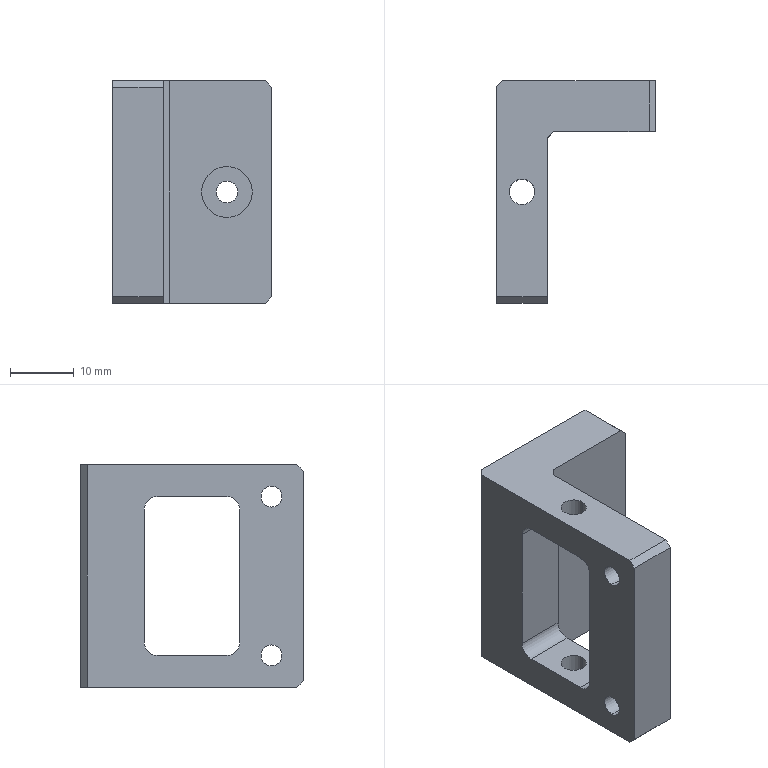Part | SolidWorks | features ICE 3, HoleWzd 2, Chamfer 1, Extrusion 1, Fillet 1 | 1 solid | 38 faces | box 25 x 35 x 35 mm | volume 11031 mm3 | plane 20 | cylinder 18 | commonest cylinder face diameters 4 x8 3.3 x4 3.4 x2 6.5 x2 8 x2
STEP:
#1=CARTESIAN_POINT('',(18.,31.6,-3.25));
#2=VERTEX_POINT('',#1);
#3=CARTESIAN_POINT('',(18.,31.6,3.25));
#4=VERTEX_POINT('',#3);
#5=CARTESIAN_POINT('',(18.,31.6,0.));
#6=DIRECTION('',(0.,1.,0.));
#7=DIRECTION('',(0.,0.,1.));
#8=AXIS2_PLACEMENT_3D('',#5,#6,#7);
#9=CIRCLE('',#8,3.25);
#10=EDGE_CURVE('',#2,#4,#9,.T.);
#11=ORIENTED_EDGE('',*,*,#10,.F.);
#12=CARTESIAN_POINT('',(18.,35.,-3.25));
#13=VERTEX_POINT('',#12);
#14=CARTESIAN_POINT('',(18.,35.,-3.25));
#15=DIRECTION('',(0.,1.,0.));
#16=VECTOR('',#15,1000.);
#17=LINE('',#14,#16);
#18=EDGE_CURVE('',#2,#13,#17,.T.);
#19=ORIENTED_EDGE('',*,*,#18,.T.);
#20=CARTESIAN_POINT('',(18.,35.,3.25));
#21=VERTEX_POINT('',#20);
#22=CARTESIAN_POINT('',(18.,35.,0.));
#23=DIRECTION('',(0.,1.,0.));
#24=DIRECTION('',(0.,0.,1.));
#25=AXIS2_PLACEMENT_3D('',#22,#23,#24);
#26=CIRCLE('',#25,3.25);
#27=EDGE_CURVE('',#13,#21,#26,.T.);
#28=ORIENTED_EDGE('',*,*,#27,.T.);
#29=CARTESIAN_POINT('',(18.,35.,3.25));
#30=DIRECTION('',(0.,1.,0.));
#31=VECTOR('',#30,1000.);
#32=LINE('',#29,#31);
#33=EDGE_CURVE('',#4,#21,#32,.T.);
#34=ORIENTED_EDGE('',*,*,#33,.F.);
#35=EDGE_LOOP('',(#11,#19,#28,#34));
#36=FACE_OUTER_BOUND('',#35,.T.);
#37=CARTESIAN_POINT('',(18.,35.,0.));
#38=DIRECTION('',(0.,1.,0.));
#39=DIRECTION('',(0.,0.,1.));
#40=AXIS2_PLACEMENT_3D('',#37,#38,#39);
#41=CYLINDRICAL_SURFACE('',#40,3.25);
#42=ADVANCED_FACE('',(#36),#41,.F.);
#43=CARTESIAN_POINT('',(18.,30.,1.7));
#44=VERTEX_POINT('',#43);
#45=CARTESIAN_POINT('',(18.,30.,-1.7));
#46=VERTEX_POINT('',#45);
#47=CARTESIAN_POINT('',(18.,30.,0.));
#48=DIRECTION('',(0.,-1.,0.));
#49=DIRECTION('',(1.,0.,0.));
#50=AXIS2_PLACEMENT_3D('',#47,#48,#49);
#51=CIRCLE('',#50,1.7);
#52=EDGE_CURVE('',#44,#46,#51,.T.);
#53=ORIENTED_EDGE('',*,*,#52,.T.);
#54=CARTESIAN_POINT('',(18.,31.6,-1.7));
#55=VERTEX_POINT('',#54);
#56=CARTESIAN_POINT('',(18.,35.,-1.7));
#57=DIRECTION('',(0.,1.,0.));
#58=VECTOR('',#57,1000.);
#59=LINE('',#56,#58);
#60=EDGE_CURVE('',#46,#55,#59,.T.);
#61=ORIENTED_EDGE('',*,*,#60,.T.);
#62=CARTESIAN_POINT('',(18.,31.6,1.7));
#63=VERTEX_POINT('',#62);
#64=CARTESIAN_POINT('',(18.,31.6,0.));
#65=DIRECTION('',(0.,1.,0.));
#66=DIRECTION('',(0.,0.,1.));
#67=AXIS2_PLACEMENT_3D('',#64,#65,#66);
#68=CIRCLE('',#67,1.7);
#69=EDGE_CURVE('',#55,#63,#68,.T.);
#70=ORIENTED_EDGE('',*,*,#69,.T.);
#71=CARTESIAN_POINT('',(18.,35.,1.7));
#72=DIRECTION('',(0.,1.,0.));
#73=VECTOR('',#72,1000.);
#74=LINE('',#71,#73);
#75=EDGE_CURVE('',#44,#63,#74,.T.);
#76=ORIENTED_EDGE('',*,*,#75,.F.);
#77=EDGE_LOOP('',(#53,#61,#70,#76));
#78=FACE_OUTER_BOUND('',#77,.T.);
#79=CARTESIAN_POINT('',(18.,35.,0.));
#80=DIRECTION('',(0.,1.,0.));
#81=DIRECTION('',(0.,0.,1.));
#82=AXIS2_PLACEMENT_3D('',#79,#80,#81);
#83=CYLINDRICAL_SURFACE('',#82,1.7);
#84=ADVANCED_FACE('',(#78),#83,.F.);
#85=CARTESIAN_POINT('',(14.,30.,0.));
#86=VERTEX_POINT('',#85);
#87=CARTESIAN_POINT('',(22.,30.,0.));
#88=VERTEX_POINT('',#87);
#89=CARTESIAN_POINT('',(18.,30.,0.));
#90=DIRECTION('',(0.,-1.,0.));
#91=DIRECTION('',(1.,0.,0.));
#92=AXIS2_PLACEMENT_3D('',#89,#90,#91);
#93=CIRCLE('',#92,4.);
#94=EDGE_CURVE('',#86,#88,#93,.T.);
#95=ORIENTED_EDGE('',*,*,#94,.F.);
#96=CARTESIAN_POINT('',(14.,27.,0.));
#97=VERTEX_POINT('',#96);
#98=CARTESIAN_POINT('',(14.,30.,0.));
#99=DIRECTION('',(0.,-1.,0.));
#100=VECTOR('',#99,1000.);
#101=LINE('',#98,#100);
#102=EDGE_CURVE('',#86,#97,#101,.T.);
#103=ORIENTED_EDGE('',*,*,#102,.T.);
#104=CARTESIAN_POINT('',(22.,27.,0.));
#105=VERTEX_POINT('',#104);
#106=CARTESIAN_POINT('',(18.,27.,0.));
#107=DIRECTION('',(0.,-1.,0.));
#108=DIRECTION('',(1.,0.,0.));
#109=AXIS2_PLACEMENT_3D('',#106,#107,#108);
#110=CIRCLE('',#109,4.);
#111=EDGE_CURVE('',#97,#105,#110,.T.);
#112=ORIENTED_EDGE('',*,*,#111,.T.);
#113=CARTESIAN_POINT('',(22.,30.,0.));
#114=DIRECTION('',(0.,-1.,0.));
#115=VECTOR('',#114,1000.);
#116=LINE('',#113,#115);
#117=EDGE_CURVE('',#88,#105,#116,.T.);
#118=ORIENTED_EDGE('',*,*,#117,.F.);
#119=EDGE_LOOP('',(#95,#103,#112,#118));
#120=FACE_OUTER_BOUND('',#119,.T.);
#121=CARTESIAN_POINT('',(18.,30.,0.));
#122=DIRECTION('',(0.,-1.,0.));
#123=DIRECTION('',(1.,0.,0.));
#124=AXIS2_PLACEMENT_3D('',#121,#122,#123);
#125=CYLINDRICAL_SURFACE('',#124,4.);
#126=ADVANCED_FACE('',(#120),#125,.F.);
#127=CARTESIAN_POINT('',(2.,17.5,-17.5));
#128=VERTEX_POINT('',#127);
#129=CARTESIAN_POINT('',(6.,17.5,-17.5));
#130=VERTEX_POINT('',#129);
#131=CARTESIAN_POINT('',(4.,17.5,-17.5));
#132=DIRECTION('',(0.,0.,1.));
#133=DIRECTION('',(1.,0.,0.));
#134=AXIS2_PLACEMENT_3D('',#131,#132,#133);
#135=CIRCLE('',#134,2.);
#136=EDGE_CURVE('',#128,#130,#135,.T.);
#137=ORIENTED_EDGE('',*,*,#136,.F.);
#138=CARTESIAN_POINT('',(2.,17.5,-12.5));
#139=VERTEX_POINT('',#138);
#140=CARTESIAN_POINT('',(2.,17.5,-17.5));
#141=DIRECTION('',(0.,0.,1.));
#142=VECTOR('',#141,1000.);
#143=LINE('',#140,#142);
#144=EDGE_CURVE('',#128,#139,#143,.T.);
#145=ORIENTED_EDGE('',*,*,#144,.T.);
#146=CARTESIAN_POINT('',(6.,17.5,-12.5));
#147=VERTEX_POINT('',#146);
#148=CARTESIAN_POINT('',(4.,17.5,-12.5));
#149=DIRECTION('',(0.,0.,-1.));
#150=DIRECTION('',(-1.,0.,0.));
#151=AXIS2_PLACEMENT_3D('',#148,#149,#150);
#152=CIRCLE('',#151,2.);
#153=EDGE_CURVE('',#147,#139,#152,.T.);
#154=ORIENTED_EDGE('',*,*,#153,.F.);
#155=CARTESIAN_POINT('',(6.,17.5,-17.5));
#156=DIRECTION('',(0.,0.,1.));
#157=VECTOR('',#156,1000.);
#158=LINE('',#155,#157);
#159=EDGE_CURVE('',#130,#147,#158,.T.);
#160=ORIENTED_EDGE('',*,*,#159,.F.);
#161=EDGE_LOOP('',(#137,#145,#154,#160));
#162=FACE_OUTER_BOUND('',#161,.T.);
#163=CARTESIAN_POINT('',(4.,17.5,-17.5));
#164=DIRECTION('',(0.,0.,1.));
#165=DIRECTION('',(1.,0.,0.));
#166=AXIS2_PLACEMENT_3D('',#163,#164,#165);
#167=CYLINDRICAL_SURFACE('',#166,2.);
#168=ADVANCED_FACE('',(#162),#167,.F.);
#169=CARTESIAN_POINT('',(2.,17.5,12.5));
#170=VERTEX_POINT('',#169);
#171=CARTESIAN_POINT('',(6.,17.5,12.5));
#172=VERTEX_POINT('',#171);
#173=CARTESIAN_POINT('',(4.,17.5,12.5));
#174=DIRECTION('',(0.,0.,1.));
#175=DIRECTION('',(0.,-1.,0.));
#176=AXIS2_PLACEMENT_3D('',#173,#174,#175);
#177=CIRCLE('',#176,2.);
#178=EDGE_CURVE('',#170,#172,#177,.T.);
#179=ORIENTED_EDGE('',*,*,#178,.F.);
#180=CARTESIAN_POINT('',(2.,17.5,17.5));
#181=VERTEX_POINT('',#180);
#182=CARTESIAN_POINT('',(2.,17.5,-17.5));
#183=DIRECTION('',(0.,0.,1.));
#184=VECTOR('',#183,1000.);
#185=LINE('',#182,#184);
#186=EDGE_CURVE('',#170,#181,#185,.T.);
#187=ORIENTED_EDGE('',*,*,#186,.T.);
#188=CARTESIAN_POINT('',(6.,17.5,17.5));
#189=VERTEX_POINT('',#188);
#190=CARTESIAN_POINT('',(4.,17.5,17.5));
#191=DIRECTION('',(0.,0.,1.));
#192=DIRECTION('',(1.,0.,0.));
#193=AXIS2_PLACEMENT_3D('',#190,#191,#192);
#194=CIRCLE('',#193,2.);
#195=EDGE_CURVE('',#181,#189,#194,.T.);
#196=ORIENTED_EDGE('',*,*,#195,.T.);
#197=CARTESIAN_POINT('',(6.,17.5,-17.5));
#198=DIRECTION('',(0.,0.,1.));
#199=VECTOR('',#198,1000.);
#200=LINE('',#197,#199);
#201=EDGE_CURVE('',#172,#189,#200,.T.);
#202=ORIENTED_EDGE('',*,*,#201,.F.);
#203=EDGE_LOOP('',(#179,#187,#196,#202));
#204=FACE_OUTER_BOUND('',#203,.T.);
#205=CARTESIAN_POINT('',(4.,17.5,-17.5));
#206=DIRECTION('',(0.,0.,1.));
#207=DIRECTION('',(1.,0.,0.));
#208=AXIS2_PLACEMENT_3D('',#205,#206,#207);
#209=CYLINDRICAL_SURFACE('',#208,2.);
#210=ADVANCED_FACE('',(#204),#209,.F.);
#211=CARTESIAN_POINT('',(8.,5.,-14.15));
#212=VERTEX_POINT('',#211);
#213=CARTESIAN_POINT('',(8.,5.,-10.85));
#214=VERTEX_POINT('',#213);
#215=CARTESIAN_POINT('',(8.,5.,-12.5));
#216=DIRECTION('',(-1.,0.,0.));
#217=DIRECTION('',(0.,-1.,0.));
#218=AXIS2_PLACEMENT_3D('',#215,#216,#217);
#219=CIRCLE('',#218,1.65);
#220=EDGE_CURVE('',#212,#214,#219,.T.);
#221=ORIENTED_EDGE('',*,*,#220,.F.);
#222=CARTESIAN_POINT('',(0.,5.,-14.15));
#223=VERTEX_POINT('',#222);
#224=CARTESIAN_POINT('',(0.,5.,-14.15));
#225=DIRECTION('',(-1.,0.,0.));
#226=VECTOR('',#225,1000.);
#227=LINE('',#224,#226);
#228=EDGE_CURVE('',#212,#223,#227,.T.);
#229=ORIENTED_EDGE('',*,*,#228,.T.);
#230=CARTESIAN_POINT('',(0.,5.,-10.85));
#231=VERTEX_POINT('',#230);
#232=CARTESIAN_POINT('',(0.,5.,-12.5));
#233=DIRECTION('',(-1.,0.,0.));
#234=DIRECTION('',(0.,0.,1.));
#235=AXIS2_PLACEMENT_3D('',#232,#233,#234);
#236=CIRCLE('',#235,1.65);
#237=EDGE_CURVE('',#223,#231,#236,.T.);
#238=ORIENTED_EDGE('',*,*,#237,.T.);
#239=CARTESIAN_POINT('',(0.,5.,-10.85));
#240=DIRECTION('',(-1.,0.,0.));
#241=VECTOR('',#240,1000.);
#242=LINE('',#239,#241);
#243=EDGE_CURVE('',#214,#231,#242,.T.);
#244=ORIENTED_EDGE('',*,*,#243,.F.);
#245=EDGE_LOOP('',(#221,#229,#238,#244));
#246=FACE_OUTER_BOUND('',#245,.T.);
#247=CARTESIAN_POINT('',(0.,5.,-12.5));
#248=DIRECTION('',(-1.,0.,0.));
#249=DIRECTION('',(0.,0.,1.));
#250=AXIS2_PLACEMENT_3D('',#247,#248,#249);
#251=CYLINDRICAL_SURFACE('',#250,1.65);
#252=ADVANCED_FACE('',(#246),#251,.F.);
#253=CARTESIAN_POINT('',(8.,5.,10.85));
#254=VERTEX_POINT('',#253);
#255=CARTESIAN_POINT('',(8.,5.,14.15));
#256=VERTEX_POINT('',#255);
#257=CARTESIAN_POINT('',(8.,5.,12.5));
#258=DIRECTION('',(-1.,0.,0.));
#259=DIRECTION('',(0.,-1.,0.));
#260=AXIS2_PLACEMENT_3D('',#257,#258,#259);
#261=CIRCLE('',#260,1.65);
#262=EDGE_CURVE('',#254,#256,#261,.T.);
#263=ORIENTED_EDGE('',*,*,#262,.F.);
#264=CARTESIAN_POINT('',(0.,5.,10.85));
#265=VERTEX_POINT('',#264);
#266=CARTESIAN_POINT('',(0.,5.,10.85));
#267=DIRECTION('',(-1.,0.,0.));
#268=VECTOR('',#267,1000.);
#269=LINE('',#266,#268);
#270=EDGE_CURVE('',#254,#265,#269,.T.);
#271=ORIENTED_EDGE('',*,*,#270,.T.);
#272=CARTESIAN_POINT('',(0.,5.,14.15));
#273=VERTEX_POINT('',#272);
#274=CARTESIAN_POINT('',(0.,5.,12.5));
#275=DIRECTION('',(-1.,0.,0.));
#276=DIRECTION('',(0.,0.,1.));
#277=AXIS2_PLACEMENT_3D('',#274,#275,#276);
#278=CIRCLE('',#277,1.65);
#279=EDGE_CURVE('',#265,#273,#278,.T.);
#280=ORIENTED_EDGE('',*,*,#279,.T.);
#281=CARTESIAN_POINT('',(0.,5.,14.15));
#282=DIRECTION('',(-1.,0.,0.));
#283=VECTOR('',#282,1000.);
#284=LINE('',#281,#283);
#285=EDGE_CURVE('',#256,#273,#284,.T.);
#286=ORIENTED_EDGE('',*,*,#285,.F.);
#287=EDGE_LOOP('',(#263,#271,#280,#286));
#288=FACE_OUTER_BOUND('',#287,.T.);
#289=CARTESIAN_POINT('',(0.,5.,12.5));
#290=DIRECTION('',(-1.,0.,0.));
#291=DIRECTION('',(0.,0.,1.));
#292=AXIS2_PLACEMENT_3D('',#289,#290,#291);
#293=CYLINDRICAL_SURFACE('',#292,1.65);
#294=ADVANCED_FACE('',(#288),#293,.F.);
#295=CARTESIAN_POINT('',(0.,0.,16.5));
#296=VERTEX_POINT('',#295);
#297=CARTESIAN_POINT('',(0.,0.,-16.5));
#298=VERTEX_POINT('',#297);
#299=CARTESIAN_POINT('',(0.,0.,17.5));
#300=DIRECTION('',(0.,0.,-1.));
#301=VECTOR('',#300,1000.);
#302=LINE('',#299,#301);
#303=EDGE_CURVE('',#296,#298,#302,.T.);
#304=ORIENTED_EDGE('',*,*,#303,.T.);
#305=CARTESIAN_POINT('',(8.,0.,-16.5));
#306=VERTEX_POINT('',#305);
#307=CARTESIAN_POINT('',(8.,0.,-16.5));
#308=DIRECTION('',(1.,0.,0.));
#309=VECTOR('',#308,1000.);
#310=LINE('',#307,#309);
#311=EDGE_CURVE('',#298,#306,#310,.T.);
#312=ORIENTED_EDGE('',*,*,#311,.T.);
#313=CARTESIAN_POINT('',(8.,0.,16.5));
#314=VERTEX_POINT('',#313);
#315=CARTESIAN_POINT('',(8.,0.,17.5));
#316=DIRECTION('',(0.,0.,-1.));
#317=VECTOR('',#316,1000.);
#318=LINE('',#315,#317);
#319=EDGE_CURVE('',#314,#306,#318,.T.);
#320=ORIENTED_EDGE('',*,*,#319,.F.);
#321=CARTESIAN_POINT('',(8.,0.,16.5));
#322=DIRECTION('',(-1.,0.,0.));
#323=VECTOR('',#322,1000.);
#324=LINE('',#321,#323);
#325=EDGE_CURVE('',#314,#296,#324,.T.);
#326=ORIENTED_EDGE('',*,*,#325,.T.);
#327=EDGE_LOOP('',(#304,#312,#320,#326));
#328=FACE_OUTER_BOUND('',#327,.T.);
#329=CARTESIAN_POINT('',(8.,0.,17.5));
#330=DIRECTION('',(0.,1.,0.));
#331=DIRECTION('',(-1.,0.,0.));
#332=AXIS2_PLACEMENT_3D('',#329,#330,#331);
#333=PLANE('',#332);
#334=ADVANCED_FACE('',(#328),#333,.F.);
#335=CARTESIAN_POINT('',(8.,5.,-12.5));
#336=DIRECTION('',(-1.,0.,0.));
#337=DIRECTION('',(0.,-1.,0.));
#338=AXIS2_PLACEMENT_3D('',#335,#336,#337);
#339=CIRCLE('',#338,1.65);
#340=EDGE_CURVE('',#214,#212,#339,.T.);
#341=ORIENTED_EDGE('',*,*,#340,.T.);
#342=ORIENTED_EDGE('',*,*,#220,.T.);
#343=EDGE_LOOP('',(#341,#342));
#344=FACE_BOUND('',#343,.T.);
#345=CARTESIAN_POINT('',(8.,5.,12.5));
#346=DIRECTION('',(-1.,0.,0.));
#347=DIRECTION('',(0.,-1.,0.));
#348=AXIS2_PLACEMENT_3D('',#345,#346,#347);
#349=CIRCLE('',#348,1.65);
#350=EDGE_CURVE('',#256,#254,#349,.T.);
#351=ORIENTED_EDGE('',*,*,#350,.T.);
#352=ORIENTED_EDGE('',*,*,#262,.T.);
#353=EDGE_LOOP('',(#351,#352));
#354=FACE_BOUND('',#353,.T.);
#355=CARTESIAN_POINT('',(8.,12.,12.5));
#356=VERTEX_POINT('',#355);
#357=CARTESIAN_POINT('',(8.,23.,12.5));
#358=VERTEX_POINT('',#357);
#359=CARTESIAN_POINT('',(8.,27.,12.5));
#360=DIRECTION('',(0.,1.,0.));
#361=VECTOR('',#360,1000.);
#362=LINE('',#359,#361);
#363=EDGE_CURVE('',#356,#358,#362,.T.);
#364=ORIENTED_EDGE('',*,*,#363,.T.);
#365=CARTESIAN_POINT('',(8.,25.,10.5));
#366=VERTEX_POINT('',#365);
#367=CARTESIAN_POINT('',(8.,23.,10.5));
#368=DIRECTION('',(-1.,0.,0.));
#369=DIRECTION('',(0.,-1.,0.));
#370=AXIS2_PLACEMENT_3D('',#367,#368,#369);
#371=CIRCLE('',#370,2.);
#372=EDGE_CURVE('',#358,#366,#371,.T.);
#373=ORIENTED_EDGE('',*,*,#372,.T.);
#374=CARTESIAN_POINT('',(8.,25.,-10.5));
#375=VERTEX_POINT('',#374);
#376=CARTESIAN_POINT('',(8.,25.,17.5));
#377=DIRECTION('',(0.,0.,-1.));
#378=VECTOR('',#377,1000.);
#379=LINE('',#376,#378);
#380=EDGE_CURVE('',#366,#375,#379,.T.);
#381=ORIENTED_EDGE('',*,*,#380,.T.);
#382=CARTESIAN_POINT('',(8.,23.,-12.5));
#383=VERTEX_POINT('',#382);
#384=CARTESIAN_POINT('',(8.,23.,-10.5));
#385=DIRECTION('',(-1.,0.,0.));
#386=DIRECTION('',(0.,-1.,0.));
#387=AXIS2_PLACEMENT_3D('',#384,#385,#386);
#388=CIRCLE('',#387,2.);
#389=EDGE_CURVE('',#375,#383,#388,.T.);
#390=ORIENTED_EDGE('',*,*,#389,.T.);
#391=CARTESIAN_POINT('',(8.,12.,-12.5));
#392=VERTEX_POINT('',#391);
#393=CARTESIAN_POINT('',(8.,27.,-12.5));
#394=DIRECTION('',(0.,-1.,0.));
#395=VECTOR('',#394,1000.);
#396=LINE('',#393,#395);
#397=EDGE_CURVE('',#383,#392,#396,.T.);
#398=ORIENTED_EDGE('',*,*,#397,.T.);
#399=CARTESIAN_POINT('',(8.,10.,-10.5));
#400=VERTEX_POINT('',#399);
#401=CARTESIAN_POINT('',(8.,12.,-10.5));
#402=DIRECTION('',(-1.,0.,0.));
#403=DIRECTION('',(0.,-1.,0.));
#404=AXIS2_PLACEMENT_3D('',#401,#402,#403);
#405=CIRCLE('',#404,2.);
#406=EDGE_CURVE('',#392,#400,#405,.T.);
#407=ORIENTED_EDGE('',*,*,#406,.T.);
#408=CARTESIAN_POINT('',(8.,10.,10.5));
#409=VERTEX_POINT('',#408);
#410=CARTESIAN_POINT('',(8.,10.,17.5));
#411=DIRECTION('',(0.,0.,1.));
#412=VECTOR('',#411,1000.);
#413=LINE('',#410,#412);
#414=EDGE_CURVE('',#400,#409,#413,.T.);
#415=ORIENTED_EDGE('',*,*,#414,.T.);
#416=CARTESIAN_POINT('',(8.,12.,10.5));
#417=DIRECTION('',(-1.,0.,0.));
#418=DIRECTION('',(0.,-1.,0.));
#419=AXIS2_PLACEMENT_3D('',#416,#417,#418);
#420=CIRCLE('',#419,2.);
#421=EDGE_CURVE('',#409,#356,#420,.T.);
#422=ORIENTED_EDGE('',*,*,#421,.T.);
#423=EDGE_LOOP('',(#364,#373,#381,#390,#398,#407,#415,#422));
#424=FACE_BOUND('',#423,.T.);
#425=CARTESIAN_POINT('',(8.,1.,-17.5));
#426=VERTEX_POINT('',#425);
#427=CARTESIAN_POINT('',(8.,26.,-17.5));
#428=VERTEX_POINT('',#427);
#429=CARTESIAN_POINT('',(8.,27.,-17.5));
#430=DIRECTION('',(0.,1.,0.));
#431=VECTOR('',#430,1000.);
#432=LINE('',#429,#431);
#433=EDGE_CURVE('',#426,#428,#432,.T.);
#434=ORIENTED_EDGE('',*,*,#433,.T.);
#435=CARTESIAN_POINT('',(8.,26.,17.5));
#436=VERTEX_POINT('',#435);
#437=CARTESIAN_POINT('',(8.,26.,17.5));
#438=DIRECTION('',(0.,0.,1.));
#439=VECTOR('',#438,1000.);
#440=LINE('',#437,#439);
#441=EDGE_CURVE('',#428,#436,#440,.T.);
#442=ORIENTED_EDGE('',*,*,#441,.T.);
#443=CARTESIAN_POINT('',(8.,1.,17.5));
#444=VERTEX_POINT('',#443);
#445=CARTESIAN_POINT('',(8.,27.,17.5));
#446=DIRECTION('',(0.,1.,0.));
#447=VECTOR('',#446,1000.);
#448=LINE('',#445,#447);
#449=EDGE_CURVE('',#444,#436,#448,.T.);
#450=ORIENTED_EDGE('',*,*,#449,.F.);
#451=CARTESIAN_POINT('',(8.,1.,17.5));
#452=DIRECTION('',(0.,-0.7071,-0.7071));
#453=VECTOR('',#452,1000.);
#454=LINE('',#451,#453);
#455=EDGE_CURVE('',#444,#314,#454,.T.);
#456=ORIENTED_EDGE('',*,*,#455,.T.);
#457=ORIENTED_EDGE('',*,*,#319,.T.);
#458=CARTESIAN_POINT('',(8.,0.,-16.5));
#459=DIRECTION('',(0.,0.7071,-0.7071));
#460=VECTOR('',#459,1000.);
#461=LINE('',#458,#460);
#462=EDGE_CURVE('',#306,#426,#461,.T.);
#463=ORIENTED_EDGE('',*,*,#462,.T.);
#464=EDGE_LOOP('',(#434,#442,#450,#456,#457,#463));
#465=FACE_OUTER_BOUND('',#464,.T.);
#466=CARTESIAN_POINT('',(8.,27.,17.5));
#467=DIRECTION('',(-1.,0.,0.));
#468=DIRECTION('',(0.,-1.,0.));
#469=AXIS2_PLACEMENT_3D('',#466,#467,#468);
#470=PLANE('',#469);
#471=ADVANCED_FACE('',(#344,#354,#424,#465),#470,.F.);
#472=CARTESIAN_POINT('',(18.,27.,0.));
#473=DIRECTION('',(0.,-1.,0.));
#474=DIRECTION('',(1.,0.,0.));
#475=AXIS2_PLACEMENT_3D('',#472,#473,#474);
#476=CIRCLE('',#475,4.);
#477=EDGE_CURVE('',#105,#97,#476,.T.);
#478=ORIENTED_EDGE('',*,*,#477,.F.);
#479=ORIENTED_EDGE('',*,*,#111,.F.);
#480=EDGE_LOOP('',(#478,#479));
#481=FACE_BOUND('',#480,.T.);
#482=CARTESIAN_POINT('',(9.,27.,17.5));
#483=VERTEX_POINT('',#482);
#484=CARTESIAN_POINT('',(24.,27.,17.5));
#485=VERTEX_POINT('',#484);
#486=CARTESIAN_POINT('',(25.,27.,17.5));
#487=DIRECTION('',(1.,0.,0.));
#488=VECTOR('',#487,1000.);
#489=LINE('',#486,#488);
#490=EDGE_CURVE('',#483,#485,#489,.T.);
#491=ORIENTED_EDGE('',*,*,#490,.F.);
#492=CARTESIAN_POINT('',(9.,27.,-17.5));
#493=VERTEX_POINT('',#492);
#494=CARTESIAN_POINT('',(9.,27.,-17.5));
#495=DIRECTION('',(0.,0.,-1.));
#496=VECTOR('',#495,1000.);
#497=LINE('',#494,#496);
#498=EDGE_CURVE('',#483,#493,#497,.T.);
#499=ORIENTED_EDGE('',*,*,#498,.T.);
#500=CARTESIAN_POINT('',(24.,27.,-17.5));
#501=VERTEX_POINT('',#500);
#502=CARTESIAN_POINT('',(25.,27.,-17.5));
#503=DIRECTION('',(1.,0.,0.));
#504=VECTOR('',#503,1000.);
#505=LINE('',#502,#504);
#506=EDGE_CURVE('',#493,#501,#505,.T.);
#507=ORIENTED_EDGE('',*,*,#506,.T.);
#508=CARTESIAN_POINT('',(25.,27.,-16.5));
#509=VERTEX_POINT('',#508);
#510=CARTESIAN_POINT('',(25.,27.,-16.5));
#511=DIRECTION('',(0.7071,0.,0.7071));
#512=VECTOR('',#511,1000.);
#513=LINE('',#510,#512);
#514=EDGE_CURVE('',#501,#509,#513,.T.);
#515=ORIENTED_EDGE('',*,*,#514,.T.);
#516=CARTESIAN_POINT('',(25.,27.,16.5));
#517=VERTEX_POINT('',#516);
#518=CARTESIAN_POINT('',(25.,27.,17.5));
#519=DIRECTION('',(0.,0.,-1.));
#520=VECTOR('',#519,1000.);
#521=LINE('',#518,#520);
#522=EDGE_CURVE('',#517,#509,#521,.T.);
#523=ORIENTED_EDGE('',*,*,#522,.F.);
#524=CARTESIAN_POINT('',(24.,27.,17.5));
#525=DIRECTION('',(-0.7071,0.,0.7071));
#526=VECTOR('',#525,1000.);
#527=LINE('',#524,#526);
#528=EDGE_CURVE('',#517,#485,#527,.T.);
#529=ORIENTED_EDGE('',*,*,#528,.T.);
#530=EDGE_LOOP('',(#491,#499,#507,#515,#523,#529));
#531=FACE_OUTER_BOUND('',#530,.T.);
#532=CARTESIAN_POINT('',(25.,27.,17.5));
#533=DIRECTION('',(0.,1.,0.));
#534=DIRECTION('',(-1.,0.,0.));
#535=AXIS2_PLACEMENT_3D('',#532,#533,#534);
#536=PLANE('',#535);
#537=ADVANCED_FACE('',(#481,#531),#536,.F.);
#538=CARTESIAN_POINT('',(25.,35.,16.5));
#539=VERTEX_POINT('',#538);
#540=CARTESIAN_POINT('',(25.,35.,-16.5));
#541=VERTEX_POINT('',#540);
#542=CARTESIAN_POINT('',(25.,35.,17.5));
#543=DIRECTION('',(0.,0.,-1.));
#544=VECTOR('',#543,1000.);
#545=LINE('',#542,#544);
#546=EDGE_CURVE('',#539,#541,#545,.T.);
#547=ORIENTED_EDGE('',*,*,#546,.F.);
#548=CARTESIAN_POINT('',(25.,35.,16.5));
#549=DIRECTION('',(0.,-1.,0.));
#550=VECTOR('',#549,1000.);
#551=LINE('',#548,#550);
#552=EDGE_CURVE('',#539,#517,#551,.T.);
#553=ORIENTED_EDGE('',*,*,#552,.T.);
#554=ORIENTED_EDGE('',*,*,#522,.T.);
#555=CARTESIAN_POINT('',(25.,35.,-16.5));
#556=DIRECTION('',(0.,1.,0.));
#557=VECTOR('',#556,1000.);
#558=LINE('',#555,#557);
#559=EDGE_CURVE('',#509,#541,#558,.T.);
#560=ORIENTED_EDGE('',*,*,#559,.T.);
#561=EDGE_LOOP('',(#547,#553,#554,#560));
#562=FACE_OUTER_BOUND('',#561,.T.);
#563=CARTESIAN_POINT('',(25.,35.,17.5));
#564=DIRECTION('',(-1.,0.,0.));
#565=DIRECTION('',(0.,-1.,0.));
#566=AXIS2_PLACEMENT_3D('',#563,#564,#565);
#567=PLANE('',#566);
#568=ADVANCED_FACE('',(#562),#567,.F.);
#569=CARTESIAN_POINT('',(18.,35.,0.));
#570=DIRECTION('',(0.,1.,0.));
#571=DIRECTION('',(0.,0.,1.));
#572=AXIS2_PLACEMENT_3D('',#569,#570,#571);
#573=CIRCLE('',#572,3.25);
#574=EDGE_CURVE('',#21,#13,#573,.T.);
#575=ORIENTED_EDGE('',*,*,#574,.F.);
#576=ORIENTED_EDGE('',*,*,#27,.F.);
#577=EDGE_LOOP('',(#575,#576));
#578=FACE_BOUND('',#577,.T.);
#579=CARTESIAN_POINT('',(24.,35.,-17.5));
#580=VERTEX_POINT('',#579);
#581=CARTESIAN_POINT('',(1.,35.,-17.5));
#582=VERTEX_POINT('',#581);
#583=CARTESIAN_POINT('',(0.,35.,-17.5));
#584=DIRECTION('',(-1.,0.,0.));
#585=VECTOR('',#584,1000.);
#586=LINE('',#583,#585);
#587=EDGE_CURVE('',#580,#582,#586,.T.);
#588=ORIENTED_EDGE('',*,*,#587,.T.);
#589=CARTESIAN_POINT('',(1.,35.,17.5));
#590=VERTEX_POINT('',#589);
#591=CARTESIAN_POINT('',(1.,35.,17.5));
#592=DIRECTION('',(0.,0.,1.));
#593=VECTOR('',#592,1000.);
#594=LINE('',#591,#593);
#595=EDGE_CURVE('',#582,#590,#594,.T.);
#596=ORIENTED_EDGE('',*,*,#595,.T.);
#597=CARTESIAN_POINT('',(24.,35.,17.5));
#598=VERTEX_POINT('',#597);
#599=CARTESIAN_POINT('',(0.,35.,17.5));
#600=DIRECTION('',(-1.,0.,0.));
#601=VECTOR('',#600,1000.);
#602=LINE('',#599,#601);
#603=EDGE_CURVE('',#598,#590,#602,.T.);
#604=ORIENTED_EDGE('',*,*,#603,.F.);
#605=CARTESIAN_POINT('',(24.,35.,17.5));
#606=DIRECTION('',(0.7071,0.,-0.7071));
#607=VECTOR('',#606,1000.);
#608=LINE('',#605,#607);
#609=EDGE_CURVE('',#598,#539,#608,.T.);
#610=ORIENTED_EDGE('',*,*,#609,.T.);
#611=ORIENTED_EDGE('',*,*,#546,.T.);
#612=CARTESIAN_POINT('',(25.,35.,-16.5));
#613=DIRECTION('',(-0.7071,0.,-0.7071));
#614=VECTOR('',#613,1000.);
#615=LINE('',#612,#614);
#616=EDGE_CURVE('',#541,#580,#615,.T.);
#617=ORIENTED_EDGE('',*,*,#616,.T.);
#618=EDGE_LOOP('',(#588,#596,#604,#610,#611,#617));
#619=FACE_OUTER_BOUND('',#618,.T.);
#620=CARTESIAN_POINT('',(0.,35.,17.5));
#621=DIRECTION('',(0.,-1.,0.));
#622=DIRECTION('',(0.,0.,-1.));
#623=AXIS2_PLACEMENT_3D('',#620,#621,#622);
#624=PLANE('',#623);
#625=ADVANCED_FACE('',(#578,#619),#624,.F.);
#626=CARTESIAN_POINT('',(0.,5.,-12.5));
#627=DIRECTION('',(-1.,0.,0.));
#628=DIRECTION('',(0.,0.,1.));
#629=AXIS2_PLACEMENT_3D('',#626,#627,#628);
#630=CIRCLE('',#629,1.65);
#631=EDGE_CURVE('',#231,#223,#630,.T.);
#632=ORIENTED_EDGE('',*,*,#631,.F.);
#633=ORIENTED_EDGE('',*,*,#237,.F.);
#634=EDGE_LOOP('',(#632,#633));
#635=FACE_BOUND('',#634,.T.);
#636=CARTESIAN_POINT('',(0.,5.,12.5));
#637=DIRECTION('',(-1.,0.,0.));
#638=DIRECTION('',(0.,0.,1.));
#639=AXIS2_PLACEMENT_3D('',#636,#637,#638);
#640=CIRCLE('',#639,1.65);
#641=EDGE_CURVE('',#273,#265,#640,.T.);
#642=ORIENTED_EDGE('',*,*,#641,.F.);
#643=ORIENTED_EDGE('',*,*,#279,.F.);
#644=EDGE_LOOP('',(#642,#643));
#645=FACE_BOUND('',#644,.T.);
#646=CARTESIAN_POINT('',(0.,10.,-10.5));
#647=VERTEX_POINT('',#646);
#648=CARTESIAN_POINT('',(0.,10.,10.5));
#649=VERTEX_POINT('',#648);
#650=CARTESIAN_POINT('',(0.,10.,-12.5));
#651=DIRECTION('',(0.,0.,1.));
#652=VECTOR('',#651,1000.);
#653=LINE('',#650,#652);
#654=EDGE_CURVE('',#647,#649,#653,.T.);
#655=ORIENTED_EDGE('',*,*,#654,.F.);
#656=CARTESIAN_POINT('',(0.,12.,-12.5));
#657=VERTEX_POINT('',#656);
#658=CARTESIAN_POINT('',(0.,12.,-10.5));
#659=DIRECTION('',(1.,0.,0.));
#660=DIRECTION('',(0.,0.,-1.));
#661=AXIS2_PLACEMENT_3D('',#658,#659,#660);
#662=CIRCLE('',#661,2.);
#663=EDGE_CURVE('',#647,#657,#662,.T.);
#664=ORIENTED_EDGE('',*,*,#663,.T.);
#665=CARTESIAN_POINT('',(0.,23.,-12.5));
#666=VERTEX_POINT('',#665);
#667=CARTESIAN_POINT('',(0.,25.,-12.5));
#668=DIRECTION('',(0.,-1.,0.));
#669=VECTOR('',#668,1000.);
#670=LINE('',#667,#669);
#671=EDGE_CURVE('',#666,#657,#670,.T.);
#672=ORIENTED_EDGE('',*,*,#671,.F.);
#673=CARTESIAN_POINT('',(0.,25.,-10.5));
#674=VERTEX_POINT('',#673);
#675=CARTESIAN_POINT('',(0.,23.,-10.5));
#676=DIRECTION('',(1.,0.,0.));
#677=DIRECTION('',(0.,0.,-1.));
#678=AXIS2_PLACEMENT_3D('',#675,#676,#677);
#679=CIRCLE('',#678,2.);
#680=EDGE_CURVE('',#666,#674,#679,.T.);
#681=ORIENTED_EDGE('',*,*,#680,.T.);
#682=CARTESIAN_POINT('',(0.,25.,10.5));
#683=VERTEX_POINT('',#682);
#684=CARTESIAN_POINT('',(0.,25.,-12.5));
#685=DIRECTION('',(0.,0.,-1.));
#686=VECTOR('',#685,1000.);
#687=LINE('',#684,#686);
#688=EDGE_CURVE('',#683,#674,#687,.T.);
#689=ORIENTED_EDGE('',*,*,#688,.F.);
#690=CARTESIAN_POINT('',(0.,23.,12.5));
#691=VERTEX_POINT('',#690);
#692=CARTESIAN_POINT('',(0.,23.,10.5));
#693=DIRECTION('',(1.,0.,0.));
#694=DIRECTION('',(0.,0.,-1.));
#695=AXIS2_PLACEMENT_3D('',#692,#693,#694);
#696=CIRCLE('',#695,2.);
#697=EDGE_CURVE('',#683,#691,#696,.T.);
#698=ORIENTED_EDGE('',*,*,#697,.T.);
#699=CARTESIAN_POINT('',(0.,12.,12.5));
#700=VERTEX_POINT('',#699);
#701=CARTESIAN_POINT('',(0.,25.,12.5));
#702=DIRECTION('',(0.,1.,0.));
#703=VECTOR('',#702,1000.);
#704=LINE('',#701,#703);
#705=EDGE_CURVE('',#700,#691,#704,.T.);
#706=ORIENTED_EDGE('',*,*,#705,.F.);
#707=CARTESIAN_POINT('',(0.,12.,10.5));
#708=DIRECTION('',(1.,0.,0.));
#709=DIRECTION('',(0.,0.,-1.));
#710=AXIS2_PLACEMENT_3D('',#707,#708,#709);
#711=CIRCLE('',#710,2.);
#712=EDGE_CURVE('',#700,#649,#711,.T.);
#713=ORIENTED_EDGE('',*,*,#712,.T.);
#714=EDGE_LOOP('',(#655,#664,#672,#681,#689,#698,#706,#713));
#715=FACE_BOUND('',#714,.T.);
#716=CARTESIAN_POINT('',(0.,34.,-17.5));
#717=VERTEX_POINT('',#716);
#718=CARTESIAN_POINT('',(0.,1.,-17.5));
#719=VERTEX_POINT('',#718);
#720=CARTESIAN_POINT('',(0.,0.,-17.5));
#721=DIRECTION('',(0.,-1.,0.));
#722=VECTOR('',#721,1000.);
#723=LINE('',#720,#722);
#724=EDGE_CURVE('',#717,#719,#723,.T.);
#725=ORIENTED_EDGE('',*,*,#724,.T.);
#726=CARTESIAN_POINT('',(0.,0.,-16.5));
#727=DIRECTION('',(0.,-0.7071,0.7071));
#728=VECTOR('',#727,1000.);
#729=LINE('',#726,#728);
#730=EDGE_CURVE('',#719,#298,#729,.T.);
#731=ORIENTED_EDGE('',*,*,#730,.T.);
#732=ORIENTED_EDGE('',*,*,#303,.F.);
#733=CARTESIAN_POINT('',(0.,1.,17.5));
#734=VERTEX_POINT('',#733);
#735=CARTESIAN_POINT('',(0.,1.,17.5));
#736=DIRECTION('',(0.,0.7071,0.7071));
#737=VECTOR('',#736,1000.);
#738=LINE('',#735,#737);
#739=EDGE_CURVE('',#296,#734,#738,.T.);
#740=ORIENTED_EDGE('',*,*,#739,.T.);
#741=CARTESIAN_POINT('',(0.,34.,17.5));
#742=VERTEX_POINT('',#741);
#743=CARTESIAN_POINT('',(0.,0.,17.5));
#744=DIRECTION('',(0.,-1.,0.));
#745=VECTOR('',#744,1000.);
#746=LINE('',#743,#745);
#747=EDGE_CURVE('',#742,#734,#746,.T.);
#748=ORIENTED_EDGE('',*,*,#747,.F.);
#749=CARTESIAN_POINT('',(0.,34.,17.5));
#750=DIRECTION('',(0.,0.,-1.));
#751=VECTOR('',#750,1000.);
#752=LINE('',#749,#751);
#753=EDGE_CURVE('',#742,#717,#752,.T.);
#754=ORIENTED_EDGE('',*,*,#753,.T.);
#755=EDGE_LOOP('',(#725,#731,#732,#740,#748,#754));
#756=FACE_OUTER_BOUND('',#755,.T.);
#757=CARTESIAN_POINT('',(0.,0.,17.5));
#758=DIRECTION('',(1.,0.,0.));
#759=DIRECTION('',(0.,0.,-1.));
#760=AXIS2_PLACEMENT_3D('',#757,#758,#759);
#761=PLANE('',#760);
#762=ADVANCED_FACE('',(#635,#645,#715,#756),#761,.F.);
#763=CARTESIAN_POINT('',(4.,17.5,17.5));
#764=DIRECTION('',(0.,0.,1.));
#765=DIRECTION('',(1.,0.,0.));
#766=AXIS2_PLACEMENT_3D('',#763,#764,#765);
#767=CIRCLE('',#766,2.);
#768=EDGE_CURVE('',#189,#181,#767,.T.);
#769=ORIENTED_EDGE('',*,*,#768,.F.);
#770=ORIENTED_EDGE('',*,*,#195,.F.);
#771=EDGE_LOOP('',(#769,#770));
#772=FACE_BOUND('',#771,.T.);
#773=ORIENTED_EDGE('',*,*,#747,.T.);
#774=CARTESIAN_POINT('',(0.,1.,17.5));
#775=DIRECTION('',(1.,0.,0.));
#776=VECTOR('',#775,1000.);
#777=LINE('',#774,#776);
#778=EDGE_CURVE('',#734,#444,#777,.T.);
#779=ORIENTED_EDGE('',*,*,#778,.T.);
#780=ORIENTED_EDGE('',*,*,#449,.T.);
#781=CARTESIAN_POINT('',(-9.,9.,17.5));
#782=DIRECTION('',(0.7071,0.7071,0.));
#783=VECTOR('',#782,1000.);
#784=LINE('',#781,#783);
#785=EDGE_CURVE('',#436,#483,#784,.T.);
#786=ORIENTED_EDGE('',*,*,#785,.T.);
#787=ORIENTED_EDGE('',*,*,#490,.T.);
#788=CARTESIAN_POINT('',(24.,0.,17.5));
#789=DIRECTION('',(0.,1.,0.));
#790=VECTOR('',#789,1000.);
#791=LINE('',#788,#790);
#792=EDGE_CURVE('',#485,#598,#791,.T.);
#793=ORIENTED_EDGE('',*,*,#792,.T.);
#794=ORIENTED_EDGE('',*,*,#603,.T.);
#795=CARTESIAN_POINT('',(0.,34.,17.5));
#796=DIRECTION('',(-0.7071,-0.7071,0.));
#797=VECTOR('',#796,1000.);
#798=LINE('',#795,#797);
#799=EDGE_CURVE('',#590,#742,#798,.T.);
#800=ORIENTED_EDGE('',*,*,#799,.T.);
#801=EDGE_LOOP('',(#773,#779,#780,#786,#787,#793,#794,#800));
#802=FACE_OUTER_BOUND('',#801,.T.);
#803=CARTESIAN_POINT('',(0.,0.,17.5));
#804=DIRECTION('',(0.,0.,-1.));
#805=DIRECTION('',(-1.,0.,0.));
#806=AXIS2_PLACEMENT_3D('',#803,#804,#805);
#807=PLANE('',#806);
#808=ADVANCED_FACE('',(#772,#802),#807,.F.);
#809=CARTESIAN_POINT('',(4.,17.5,-17.5));
#810=DIRECTION('',(0.,0.,1.));
#811=DIRECTION('',(1.,0.,0.));
#812=AXIS2_PLACEMENT_3D('',#809,#810,#811);
#813=CIRCLE('',#812,2.);
#814=EDGE_CURVE('',#130,#128,#813,.T.);
#815=ORIENTED_EDGE('',*,*,#814,.T.);
#816=ORIENTED_EDGE('',*,*,#136,.T.);
#817=EDGE_LOOP('',(#815,#816));
#818=FACE_BOUND('',#817,.T.);
#819=ORIENTED_EDGE('',*,*,#433,.F.);
#820=CARTESIAN_POINT('',(0.,1.,-17.5));
#821=DIRECTION('',(-1.,0.,0.));
#822=VECTOR('',#821,1000.);
#823=LINE('',#820,#822);
#824=EDGE_CURVE('',#426,#719,#823,.T.);
#825=ORIENTED_EDGE('',*,*,#824,.T.);
#826=ORIENTED_EDGE('',*,*,#724,.F.);
#827=CARTESIAN_POINT('',(-17.,17.,-17.5));
#828=DIRECTION('',(0.7071,0.7071,0.));
#829=VECTOR('',#828,1000.);
#830=LINE('',#827,#829);
#831=EDGE_CURVE('',#717,#582,#830,.T.);
#832=ORIENTED_EDGE('',*,*,#831,.T.);
#833=ORIENTED_EDGE('',*,*,#587,.F.);
#834=CARTESIAN_POINT('',(24.,27.,-17.5));
#835=DIRECTION('',(0.,-1.,0.));
#836=VECTOR('',#835,1000.);
#837=LINE('',#834,#836);
#838=EDGE_CURVE('',#580,#501,#837,.T.);
#839=ORIENTED_EDGE('',*,*,#838,.T.);
#840=ORIENTED_EDGE('',*,*,#506,.F.);
#841=CARTESIAN_POINT('',(9.,27.,-17.5));
#842=DIRECTION('',(-0.7071,-0.7071,0.));
#843=VECTOR('',#842,1000.);
#844=LINE('',#841,#843);
#845=EDGE_CURVE('',#493,#428,#844,.T.);
#846=ORIENTED_EDGE('',*,*,#845,.T.);
#847=EDGE_LOOP('',(#819,#825,#826,#832,#833,#839,#840,#846));
#848=FACE_OUTER_BOUND('',#847,.T.);
#849=CARTESIAN_POINT('',(0.,0.,-17.5));
#850=DIRECTION('',(0.,0.,-1.));
#851=DIRECTION('',(-1.,0.,0.));
#852=AXIS2_PLACEMENT_3D('',#849,#850,#851);
#853=PLANE('',#852);
#854=ADVANCED_FACE('',(#818,#848),#853,.T.);
#855=ORIENTED_EDGE('',*,*,#153,.T.);
#856=CARTESIAN_POINT('',(4.,17.5,-12.5));
#857=DIRECTION('',(0.,0.,-1.));
#858=DIRECTION('',(-1.,0.,0.));
#859=AXIS2_PLACEMENT_3D('',#856,#857,#858);
#860=CIRCLE('',#859,2.);
#861=EDGE_CURVE('',#139,#147,#860,.T.);
#862=ORIENTED_EDGE('',*,*,#861,.T.);
#863=EDGE_LOOP('',(#855,#862));
#864=FACE_BOUND('',#863,.T.);
#865=ORIENTED_EDGE('',*,*,#671,.T.);
#866=CARTESIAN_POINT('',(8.,12.,-12.5));
#867=DIRECTION('',(1.,0.,0.));
#868=VECTOR('',#867,1000.);
#869=LINE('',#866,#868);
#870=EDGE_CURVE('',#657,#392,#869,.T.);
#871=ORIENTED_EDGE('',*,*,#870,.T.);
#872=ORIENTED_EDGE('',*,*,#397,.F.);
#873=CARTESIAN_POINT('',(0.,23.,-12.5));
#874=DIRECTION('',(-1.,0.,0.));
#875=VECTOR('',#874,1000.);
#876=LINE('',#873,#875);
#877=EDGE_CURVE('',#383,#666,#876,.T.);
#878=ORIENTED_EDGE('',*,*,#877,.T.);
#879=EDGE_LOOP('',(#865,#871,#872,#878));
#880=FACE_OUTER_BOUND('',#879,.T.);
#881=CARTESIAN_POINT('',(25.,25.,-12.5));
#882=DIRECTION('',(0.,0.,-1.));
#883=DIRECTION('',(-1.,0.,0.));
#884=AXIS2_PLACEMENT_3D('',#881,#882,#883);
#885=PLANE('',#884);
#886=ADVANCED_FACE('',(#864,#880),#885,.F.);
#887=ORIENTED_EDGE('',*,*,#380,.F.);
#888=CARTESIAN_POINT('',(0.,25.,10.5));
#889=DIRECTION('',(-1.,0.,0.));
#890=VECTOR('',#889,1000.);
#891=LINE('',#888,#890);
#892=EDGE_CURVE('',#366,#683,#891,.T.);
#893=ORIENTED_EDGE('',*,*,#892,.T.);
#894=ORIENTED_EDGE('',*,*,#688,.T.);
#895=CARTESIAN_POINT('',(8.,25.,-10.5));
#896=DIRECTION('',(1.,0.,0.));
#897=VECTOR('',#896,1000.);
#898=LINE('',#895,#897);
#899=EDGE_CURVE('',#674,#375,#898,.T.);
#900=ORIENTED_EDGE('',*,*,#899,.T.);
#901=EDGE_LOOP('',(#887,#893,#894,#900));
#902=FACE_OUTER_BOUND('',#901,.T.);
#903=CARTESIAN_POINT('',(25.,25.,-12.5));
#904=DIRECTION('',(0.,1.,0.));
#905=DIRECTION('',(0.,0.,1.));
#906=AXIS2_PLACEMENT_3D('',#903,#904,#905);
#907=PLANE('',#906);
#908=ADVANCED_FACE('',(#902),#907,.F.);
#909=CARTESIAN_POINT('',(4.,17.5,12.5));
#910=DIRECTION('',(0.,0.,1.));
#911=DIRECTION('',(0.,-1.,0.));
#912=AXIS2_PLACEMENT_3D('',#909,#910,#911);
#913=CIRCLE('',#912,2.);
#914=EDGE_CURVE('',#172,#170,#913,.T.);
#915=ORIENTED_EDGE('',*,*,#914,.T.);
#916=ORIENTED_EDGE('',*,*,#178,.T.);
#917=EDGE_LOOP('',(#915,#916));
#918=FACE_BOUND('',#917,.T.);
#919=ORIENTED_EDGE('',*,*,#363,.F.);
#920=CARTESIAN_POINT('',(0.,12.,12.5));
#921=DIRECTION('',(-1.,0.,0.));
#922=VECTOR('',#921,1000.);
#923=LINE('',#920,#922);
#924=EDGE_CURVE('',#356,#700,#923,.T.);
#925=ORIENTED_EDGE('',*,*,#924,.T.);
#926=ORIENTED_EDGE('',*,*,#705,.T.);
#927=CARTESIAN_POINT('',(8.,23.,12.5));
#928=DIRECTION('',(1.,0.,0.));
#929=VECTOR('',#928,1000.);
#930=LINE('',#927,#929);
#931=EDGE_CURVE('',#691,#358,#930,.T.);
#932=ORIENTED_EDGE('',*,*,#931,.T.);
#933=EDGE_LOOP('',(#919,#925,#926,#932));
#934=FACE_OUTER_BOUND('',#933,.T.);
#935=CARTESIAN_POINT('',(25.,25.,12.5));
#936=DIRECTION('',(0.,0.,1.));
#937=DIRECTION('',(0.,-1.,0.));
#938=AXIS2_PLACEMENT_3D('',#935,#936,#937);
#939=PLANE('',#938);
#940=ADVANCED_FACE('',(#918,#934),#939,.F.);
#941=ORIENTED_EDGE('',*,*,#414,.F.);
#942=CARTESIAN_POINT('',(0.,10.,-10.5));
#943=DIRECTION('',(-1.,0.,0.));
#944=VECTOR('',#943,1000.);
#945=LINE('',#942,#944);
#946=EDGE_CURVE('',#400,#647,#945,.T.);
#947=ORIENTED_EDGE('',*,*,#946,.T.);
#948=ORIENTED_EDGE('',*,*,#654,.T.);
#949=CARTESIAN_POINT('',(8.,10.,10.5));
#950=DIRECTION('',(1.,0.,0.));
#951=VECTOR('',#950,1000.);
#952=LINE('',#949,#951);
#953=EDGE_CURVE('',#649,#409,#952,.T.);
#954=ORIENTED_EDGE('',*,*,#953,.T.);
#955=EDGE_LOOP('',(#941,#947,#948,#954));
#956=FACE_OUTER_BOUND('',#955,.T.);
#957=CARTESIAN_POINT('',(25.,10.,-12.5));
#958=DIRECTION('',(0.,-1.,0.));
#959=DIRECTION('',(0.,0.,-1.));
#960=AXIS2_PLACEMENT_3D('',#957,#958,#959);
#961=PLANE('',#960);
#962=ADVANCED_FACE('',(#956),#961,.F.);
#963=ORIENTED_EDGE('',*,*,#270,.F.);
#964=ORIENTED_EDGE('',*,*,#350,.F.);
#965=ORIENTED_EDGE('',*,*,#285,.T.);
#966=ORIENTED_EDGE('',*,*,#641,.T.);
#967=EDGE_LOOP('',(#963,#964,#965,#966));
#968=FACE_OUTER_BOUND('',#967,.T.);
#969=CARTESIAN_POINT('',(0.,5.,12.5));
#970=DIRECTION('',(-1.,0.,0.));
#971=DIRECTION('',(0.,0.,1.));
#972=AXIS2_PLACEMENT_3D('',#969,#970,#971);
#973=CYLINDRICAL_SURFACE('',#972,1.65);
#974=ADVANCED_FACE('',(#968),#973,.F.);
#975=ORIENTED_EDGE('',*,*,#228,.F.);
#976=ORIENTED_EDGE('',*,*,#340,.F.);
#977=ORIENTED_EDGE('',*,*,#243,.T.);
#978=ORIENTED_EDGE('',*,*,#631,.T.);
#979=EDGE_LOOP('',(#975,#976,#977,#978));
#980=FACE_OUTER_BOUND('',#979,.T.);
#981=CARTESIAN_POINT('',(0.,5.,-12.5));
#982=DIRECTION('',(-1.,0.,0.));
#983=DIRECTION('',(0.,0.,1.));
#984=AXIS2_PLACEMENT_3D('',#981,#982,#983);
#985=CYLINDRICAL_SURFACE('',#984,1.65);
#986=ADVANCED_FACE('',(#980),#985,.F.);
#987=ORIENTED_EDGE('',*,*,#186,.F.);
#988=ORIENTED_EDGE('',*,*,#914,.F.);
#989=ORIENTED_EDGE('',*,*,#201,.T.);
#990=ORIENTED_EDGE('',*,*,#768,.T.);
#991=EDGE_LOOP('',(#987,#988,#989,#990));
#992=FACE_OUTER_BOUND('',#991,.T.);
#993=CARTESIAN_POINT('',(4.,17.5,-17.5));
#994=DIRECTION('',(0.,0.,1.));
#995=DIRECTION('',(1.,0.,0.));
#996=AXIS2_PLACEMENT_3D('',#993,#994,#995);
#997=CYLINDRICAL_SURFACE('',#996,2.);
#998=ADVANCED_FACE('',(#992),#997,.F.);
#999=ORIENTED_EDGE('',*,*,#144,.F.);
#1000=ORIENTED_EDGE('',*,*,#814,.F.);
#1001=ORIENTED_EDGE('',*,*,#159,.T.);
#1002=ORIENTED_EDGE('',*,*,#861,.F.);
#1003=EDGE_LOOP('',(#999,#1000,#1001,#1002));
#1004=FACE_OUTER_BOUND('',#1003,.T.);
#1005=CARTESIAN_POINT('',(4.,17.5,-17.5));
#1006=DIRECTION('',(0.,0.,1.));
#1007=DIRECTION('',(1.,0.,0.));
#1008=AXIS2_PLACEMENT_3D('',#1005,#1006,#1007);
#1009=CYLINDRICAL_SURFACE('',#1008,2.);
#1010=ADVANCED_FACE('',(#1004),#1009,.F.);
#1011=ORIENTED_EDGE('',*,*,#406,.F.);
#1012=ORIENTED_EDGE('',*,*,#870,.F.);
#1013=ORIENTED_EDGE('',*,*,#663,.F.);
#1014=ORIENTED_EDGE('',*,*,#946,.F.);
#1015=EDGE_LOOP('',(#1011,#1012,#1013,#1014));
#1016=FACE_OUTER_BOUND('',#1015,.T.);
#1017=CARTESIAN_POINT('',(25.,12.,-10.5));
#1018=DIRECTION('',(1.,0.,0.));
#1019=DIRECTION('',(0.,0.,-1.));
#1020=AXIS2_PLACEMENT_3D('',#1017,#1018,#1019);
#1021=CYLINDRICAL_SURFACE('',#1020,2.);
#1022=ADVANCED_FACE('',(#1016),#1021,.F.);
#1023=ORIENTED_EDGE('',*,*,#421,.F.);
#1024=ORIENTED_EDGE('',*,*,#953,.F.);
#1025=ORIENTED_EDGE('',*,*,#712,.F.);
#1026=ORIENTED_EDGE('',*,*,#924,.F.);
#1027=EDGE_LOOP('',(#1023,#1024,#1025,#1026));
#1028=FACE_OUTER_BOUND('',#1027,.T.);
#1029=CARTESIAN_POINT('',(25.,12.,10.5));
#1030=DIRECTION('',(1.,0.,0.));
#1031=DIRECTION('',(0.,0.,-1.));
#1032=AXIS2_PLACEMENT_3D('',#1029,#1030,#1031);
#1033=CYLINDRICAL_SURFACE('',#1032,2.);
#1034=ADVANCED_FACE('',(#1028),#1033,.F.);
#1035=ORIENTED_EDGE('',*,*,#372,.F.);
#1036=ORIENTED_EDGE('',*,*,#931,.F.);
#1037=ORIENTED_EDGE('',*,*,#697,.F.);
#1038=ORIENTED_EDGE('',*,*,#892,.F.);
#1039=EDGE_LOOP('',(#1035,#1036,#1037,#1038));
#1040=FACE_OUTER_BOUND('',#1039,.T.);
#1041=CARTESIAN_POINT('',(25.,23.,10.5));
#1042=DIRECTION('',(1.,0.,0.));
#1043=DIRECTION('',(0.,0.,-1.));
#1044=AXIS2_PLACEMENT_3D('',#1041,#1042,#1043);
#1045=CYLINDRICAL_SURFACE('',#1044,2.);
#1046=ADVANCED_FACE('',(#1040),#1045,.F.);
#1047=ORIENTED_EDGE('',*,*,#389,.F.);
#1048=ORIENTED_EDGE('',*,*,#899,.F.);
#1049=ORIENTED_EDGE('',*,*,#680,.F.);
#1050=ORIENTED_EDGE('',*,*,#877,.F.);
#1051=EDGE_LOOP('',(#1047,#1048,#1049,#1050));
#1052=FACE_OUTER_BOUND('',#1051,.T.);
#1053=CARTESIAN_POINT('',(25.,23.,-10.5));
#1054=DIRECTION('',(1.,0.,0.));
#1055=DIRECTION('',(0.,0.,-1.));
#1056=AXIS2_PLACEMENT_3D('',#1053,#1054,#1055);
#1057=CYLINDRICAL_SURFACE('',#1056,2.);
#1058=ADVANCED_FACE('',(#1052),#1057,.F.);
#1059=ORIENTED_EDGE('',*,*,#102,.F.);
#1060=CARTESIAN_POINT('',(18.,30.,0.));
#1061=DIRECTION('',(0.,-1.,0.));
#1062=DIRECTION('',(1.,0.,0.));
#1063=AXIS2_PLACEMENT_3D('',#1060,#1061,#1062);
#1064=CIRCLE('',#1063,4.);
#1065=EDGE_CURVE('',#88,#86,#1064,.T.);
#1066=ORIENTED_EDGE('',*,*,#1065,.F.);
#1067=ORIENTED_EDGE('',*,*,#117,.T.);
#1068=ORIENTED_EDGE('',*,*,#477,.T.);
#1069=EDGE_LOOP('',(#1059,#1066,#1067,#1068));
#1070=FACE_OUTER_BOUND('',#1069,.T.);
#1071=CARTESIAN_POINT('',(18.,30.,0.));
#1072=DIRECTION('',(0.,-1.,0.));
#1073=DIRECTION('',(1.,0.,0.));
#1074=AXIS2_PLACEMENT_3D('',#1071,#1072,#1073);
#1075=CYLINDRICAL_SURFACE('',#1074,4.);
#1076=ADVANCED_FACE('',(#1070),#1075,.F.);
#1077=ORIENTED_EDGE('',*,*,#52,.F.);
#1078=CARTESIAN_POINT('',(18.,30.,0.));
#1079=DIRECTION('',(0.,-1.,0.));
#1080=DIRECTION('',(1.,0.,0.));
#1081=AXIS2_PLACEMENT_3D('',#1078,#1079,#1080);
#1082=CIRCLE('',#1081,1.7);
#1083=EDGE_CURVE('',#46,#44,#1082,.T.);
#1084=ORIENTED_EDGE('',*,*,#1083,.F.);
#1085=EDGE_LOOP('',(#1077,#1084));
#1086=FACE_BOUND('',#1085,.T.);
#1087=ORIENTED_EDGE('',*,*,#1065,.T.);
#1088=ORIENTED_EDGE('',*,*,#94,.T.);
#1089=EDGE_LOOP('',(#1087,#1088));
#1090=FACE_OUTER_BOUND('',#1089,.T.);
#1091=CARTESIAN_POINT('',(18.,30.,0.));
#1092=DIRECTION('',(0.,-1.,0.));
#1093=DIRECTION('',(1.,0.,0.));
#1094=AXIS2_PLACEMENT_3D('',#1091,#1092,#1093);
#1095=PLANE('',#1094);
#1096=ADVANCED_FACE('',(#1086,#1090),#1095,.T.);
#1097=ORIENTED_EDGE('',*,*,#785,.F.);
#1098=ORIENTED_EDGE('',*,*,#441,.F.);
#1099=ORIENTED_EDGE('',*,*,#845,.F.);
#1100=ORIENTED_EDGE('',*,*,#498,.F.);
#1101=EDGE_LOOP('',(#1097,#1098,#1099,#1100));
#1102=FACE_OUTER_BOUND('',#1101,.T.);
#1103=CARTESIAN_POINT('',(9.,27.,17.5));
#1104=DIRECTION('',(0.7071,-0.7071,0.));
#1105=DIRECTION('',(0.7071,0.7071,0.));
#1106=AXIS2_PLACEMENT_3D('',#1103,#1104,#1105);
#1107=PLANE('',#1106);
#1108=ADVANCED_FACE('',(#1102),#1107,.T.);
#1109=ORIENTED_EDGE('',*,*,#730,.F.);
#1110=ORIENTED_EDGE('',*,*,#824,.F.);
#1111=ORIENTED_EDGE('',*,*,#462,.F.);
#1112=ORIENTED_EDGE('',*,*,#311,.F.);
#1113=EDGE_LOOP('',(#1109,#1110,#1111,#1112));
#1114=FACE_OUTER_BOUND('',#1113,.T.);
#1115=CARTESIAN_POINT('',(8.,0.,-16.5));
#1116=DIRECTION('',(0.,-0.7071,-0.7071));
#1117=DIRECTION('',(0.,0.7071,-0.7071));
#1118=AXIS2_PLACEMENT_3D('',#1115,#1116,#1117);
#1119=PLANE('',#1118);
#1120=ADVANCED_FACE('',(#1114),#1119,.T.);
#1121=ORIENTED_EDGE('',*,*,#739,.F.);
#1122=ORIENTED_EDGE('',*,*,#325,.F.);
#1123=ORIENTED_EDGE('',*,*,#455,.F.);
#1124=ORIENTED_EDGE('',*,*,#778,.F.);
#1125=EDGE_LOOP('',(#1121,#1122,#1123,#1124));
#1126=FACE_OUTER_BOUND('',#1125,.T.);
#1127=CARTESIAN_POINT('',(0.,1.,17.5));
#1128=DIRECTION('',(0.,0.7071,-0.7071));
#1129=DIRECTION('',(0.,0.7071,0.7071));
#1130=AXIS2_PLACEMENT_3D('',#1127,#1128,#1129);
#1131=PLANE('',#1130);
#1132=ADVANCED_FACE('',(#1126),#1131,.F.);
#1133=ORIENTED_EDGE('',*,*,#799,.F.);
#1134=ORIENTED_EDGE('',*,*,#595,.F.);
#1135=ORIENTED_EDGE('',*,*,#831,.F.);
#1136=ORIENTED_EDGE('',*,*,#753,.F.);
#1137=EDGE_LOOP('',(#1133,#1134,#1135,#1136));
#1138=FACE_OUTER_BOUND('',#1137,.T.);
#1139=CARTESIAN_POINT('',(0.,34.,17.5));
#1140=DIRECTION('',(0.7071,-0.7071,0.));
#1141=DIRECTION('',(0.7071,0.7071,0.));
#1142=AXIS2_PLACEMENT_3D('',#1139,#1140,#1141);
#1143=PLANE('',#1142);
#1144=ADVANCED_FACE('',(#1138),#1143,.F.);
#1145=ORIENTED_EDGE('',*,*,#528,.F.);
#1146=ORIENTED_EDGE('',*,*,#552,.F.);
#1147=ORIENTED_EDGE('',*,*,#609,.F.);
#1148=ORIENTED_EDGE('',*,*,#792,.F.);
#1149=EDGE_LOOP('',(#1145,#1146,#1147,#1148));
#1150=FACE_OUTER_BOUND('',#1149,.T.);
#1151=CARTESIAN_POINT('',(24.,0.,17.5));
#1152=DIRECTION('',(-0.7071,0.,-0.7071));
#1153=DIRECTION('',(-0.7071,0.,0.7071));
#1154=AXIS2_PLACEMENT_3D('',#1151,#1152,#1153);
#1155=PLANE('',#1154);
#1156=ADVANCED_FACE('',(#1150),#1155,.F.);
#1157=ORIENTED_EDGE('',*,*,#514,.F.);
#1158=ORIENTED_EDGE('',*,*,#838,.F.);
#1159=ORIENTED_EDGE('',*,*,#616,.F.);
#1160=ORIENTED_EDGE('',*,*,#559,.F.);
#1161=EDGE_LOOP('',(#1157,#1158,#1159,#1160));
#1162=FACE_OUTER_BOUND('',#1161,.T.);
#1163=CARTESIAN_POINT('',(25.,35.,-16.5));
#1164=DIRECTION('',(0.7071,0.,-0.7071));
#1165=DIRECTION('',(-0.7071,0.,-0.7071));
#1166=AXIS2_PLACEMENT_3D('',#1163,#1164,#1165);
#1167=PLANE('',#1166);
#1168=ADVANCED_FACE('',(#1162),#1167,.T.);
#1169=ORIENTED_EDGE('',*,*,#60,.F.);
#1170=ORIENTED_EDGE('',*,*,#1083,.T.);
#1171=ORIENTED_EDGE('',*,*,#75,.T.);
#1172=CARTESIAN_POINT('',(18.,31.6,0.));
#1173=DIRECTION('',(0.,1.,0.));
#1174=DIRECTION('',(0.,0.,1.));
#1175=AXIS2_PLACEMENT_3D('',#1172,#1173,#1174);
#1176=CIRCLE('',#1175,1.7);
#1177=EDGE_CURVE('',#63,#55,#1176,.T.);
#1178=ORIENTED_EDGE('',*,*,#1177,.T.);
#1179=EDGE_LOOP('',(#1169,#1170,#1171,#1178));
#1180=FACE_OUTER_BOUND('',#1179,.T.);
#1181=CARTESIAN_POINT('',(18.,35.,0.));
#1182=DIRECTION('',(0.,1.,0.));
#1183=DIRECTION('',(0.,0.,1.));
#1184=AXIS2_PLACEMENT_3D('',#1181,#1182,#1183);
#1185=CYLINDRICAL_SURFACE('',#1184,1.7);
#1186=ADVANCED_FACE('',(#1180),#1185,.F.);
#1187=ORIENTED_EDGE('',*,*,#1177,.F.);
#1188=ORIENTED_EDGE('',*,*,#69,.F.);
#1189=EDGE_LOOP('',(#1187,#1188));
#1190=FACE_BOUND('',#1189,.T.);
#1191=CARTESIAN_POINT('',(18.,31.6,0.));
#1192=DIRECTION('',(0.,1.,0.));
#1193=DIRECTION('',(0.,0.,1.));
#1194=AXIS2_PLACEMENT_3D('',#1191,#1192,#1193);
#1195=CIRCLE('',#1194,3.25);
#1196=EDGE_CURVE('',#4,#2,#1195,.T.);
#1197=ORIENTED_EDGE('',*,*,#1196,.T.);
#1198=ORIENTED_EDGE('',*,*,#10,.T.);
#1199=EDGE_LOOP('',(#1197,#1198));
#1200=FACE_OUTER_BOUND('',#1199,.T.);
#1201=CARTESIAN_POINT('',(19.7,31.6,0.));
#1202=DIRECTION('',(0.,-1.,0.));
#1203=DIRECTION('',(0.,0.,-1.));
#1204=AXIS2_PLACEMENT_3D('',#1201,#1202,#1203);
#1205=PLANE('',#1204);
#1206=ADVANCED_FACE('',(#1190,#1200),#1205,.F.);
#1207=ORIENTED_EDGE('',*,*,#18,.F.);
#1208=ORIENTED_EDGE('',*,*,#1196,.F.);
#1209=ORIENTED_EDGE('',*,*,#33,.T.);
#1210=ORIENTED_EDGE('',*,*,#574,.T.);
#1211=EDGE_LOOP('',(#1207,#1208,#1209,#1210));
#1212=FACE_OUTER_BOUND('',#1211,.T.);
#1213=CARTESIAN_POINT('',(18.,35.,0.));
#1214=DIRECTION('',(0.,1.,0.));
#1215=DIRECTION('',(0.,0.,1.));
#1216=AXIS2_PLACEMENT_3D('',#1213,#1214,#1215);
#1217=CYLINDRICAL_SURFACE('',#1216,3.25);
#1218=ADVANCED_FACE('',(#1212),#1217,.F.);
#1219=CLOSED_SHELL('',(#42,#84,#126,#168,#210,#252,#294,#334,#471,#537,#568,#625,#762,#808,#854,#886,#908,#940,#962,#974,#986,#998,#1010,#1022,#1034,#1046,#1058,#1076,#1096,#1108,#1120,#1132,#1144,#1156,#1168,#1186,#1206,#1218));
#1220=MANIFOLD_SOLID_BREP('',#1219);
#1221=CARTESIAN_POINT('',(0.,0.,0.));
#1222=DIRECTION('',(0.,0.,1.));
#1223=DIRECTION('',(1.,0.,0.));
#1224=AXIS2_PLACEMENT_3D('',#1221,#1222,#1223);
#1225=(LENGTH_UNIT()NAMED_UNIT(*)SI_UNIT(.MILLI.,.METRE.));
#1226=UNCERTAINTY_MEASURE_WITH_UNIT(LENGTH_MEASURE(0.00001),#1225,'','');
#1227=(NAMED_UNIT(*)PLANE_ANGLE_UNIT()SI_UNIT($,.RADIAN.));
#1228=(NAMED_UNIT(*)SI_UNIT($,.STERADIAN.)SOLID_ANGLE_UNIT());
#1229=(GEOMETRIC_REPRESENTATION_CONTEXT(3)GLOBAL_UNCERTAINTY_ASSIGNED_CONTEXT((#1226))GLOBAL_UNIT_ASSIGNED_CONTEXT((#1225,#1227,#1228))REPRESENTATION_CONTEXT('',''));
#1230=ADVANCED_BREP_SHAPE_REPRESENTATION('',(#1220,#1224),#1229);